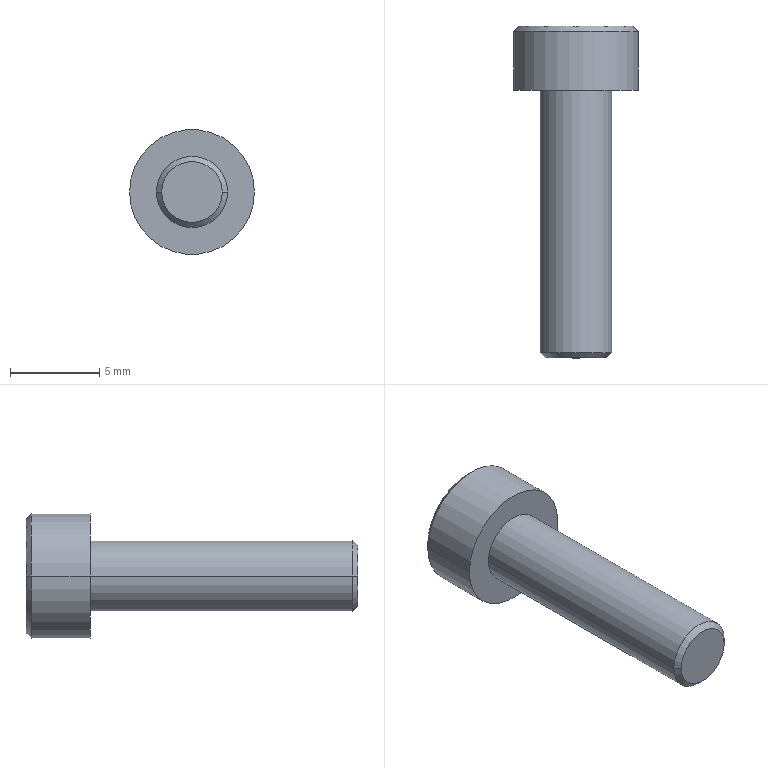Part | NX | 1 solid | 56 faces | box 7 x 18.6 x 7 mm | volume 309.592 mm3 | plane 44 | cone 6 | cylinder 6 | commonest cylinder face diameters 3 x2 4 x2 7 x2
STEP:
#1=CARTESIAN_POINT('',(1.7,-15.,0.));
#2=VERTEX_POINT('',#1);
#3=CARTESIAN_POINT('',(-1.7,-15.,0.));
#4=VERTEX_POINT('',#3);
#5=CARTESIAN_POINT('',(0.,-15.,0.));
#6=DIRECTION('',(0.,1.,0.));
#7=DIRECTION('',(-1.,0.,0.));
#8=AXIS2_PLACEMENT_3D('',#5,#6,#7);
#9=CIRCLE('',#8,1.7);
#10=EDGE_CURVE('',#2,#4,#9,.T.);
#11=ORIENTED_EDGE('',*,*,#10,.F.);
#12=CARTESIAN_POINT('',(0.,-15.,0.));
#13=DIRECTION('',(0.,1.,0.));
#14=DIRECTION('',(-1.,0.,0.));
#15=AXIS2_PLACEMENT_3D('',#12,#13,#14);
#16=CIRCLE('',#15,1.7);
#17=EDGE_CURVE('',#4,#2,#16,.T.);
#18=ORIENTED_EDGE('',*,*,#17,.F.);
#19=EDGE_LOOP('',(#11,#18));
#20=FACE_BOUND('',#19,.T.);
#21=CARTESIAN_POINT('',(0.,-15.,0.));
#22=DIRECTION('',(0.,-1.,0.));
#23=DIRECTION('',(0.,0.,-1.));
#24=AXIS2_PLACEMENT_3D('',#21,#22,#23);
#25=PLANE('',#24);
#26=ADVANCED_FACE('',(#20),#25,.T.);
#27=ORIENTED_EDGE('',*,*,#10,.T.);
#28=CARTESIAN_POINT('',(-2.,-14.7,0.));
#29=VERTEX_POINT('',#28);
#30=CARTESIAN_POINT('',(-1.85,-14.85,0.));
#31=DIRECTION('',(-0.7071,0.7071,0.));
#32=VECTOR('',#31,1000.);
#33=LINE('',#30,#32);
#34=EDGE_CURVE('',#29,#4,#33,.F.);
#35=ORIENTED_EDGE('',*,*,#34,.F.);
#36=CARTESIAN_POINT('',(2.,-14.7,0.));
#37=VERTEX_POINT('',#36);
#38=CARTESIAN_POINT('',(0.,-14.7,0.));
#39=DIRECTION('',(0.,1.,0.));
#40=DIRECTION('',(-1.,0.,0.));
#41=AXIS2_PLACEMENT_3D('',#38,#39,#40);
#42=CIRCLE('',#41,2.);
#43=EDGE_CURVE('',#37,#29,#42,.T.);
#44=ORIENTED_EDGE('',*,*,#43,.F.);
#45=CARTESIAN_POINT('',(1.85,-14.85,0.));
#46=DIRECTION('',(0.7071,0.7071,0.));
#47=VECTOR('',#46,1000.);
#48=LINE('',#45,#47);
#49=EDGE_CURVE('',#37,#2,#48,.F.);
#50=ORIENTED_EDGE('',*,*,#49,.T.);
#51=EDGE_LOOP('',(#27,#35,#44,#50));
#52=FACE_BOUND('',#51,.T.);
#53=CARTESIAN_POINT('',(0.,-14.85,0.));
#54=DIRECTION('',(0.,1.,0.));
#55=DIRECTION('',(1.,0.,0.));
#56=AXIS2_PLACEMENT_3D('',#53,#54,#55);
#57=CONICAL_SURFACE('',#56,1.85,0.7854);
#58=ADVANCED_FACE('',(#52),#57,.T.);
#59=CARTESIAN_POINT('',(0.,-14.7,0.));
#60=DIRECTION('',(0.,1.,0.));
#61=DIRECTION('',(-1.,0.,0.));
#62=AXIS2_PLACEMENT_3D('',#59,#60,#61);
#63=CIRCLE('',#62,2.);
#64=EDGE_CURVE('',#29,#37,#63,.T.);
#65=ORIENTED_EDGE('',*,*,#64,.T.);
#66=CARTESIAN_POINT('',(2.,0.,0.));
#67=VERTEX_POINT('',#66);
#68=CARTESIAN_POINT('',(2.,4.53,0.));
#69=DIRECTION('',(0.,-1.,0.));
#70=VECTOR('',#69,1000.);
#71=LINE('',#68,#70);
#72=EDGE_CURVE('',#67,#37,#71,.T.);
#73=ORIENTED_EDGE('',*,*,#72,.F.);
#74=CARTESIAN_POINT('',(-2.,0.,0.));
#75=VERTEX_POINT('',#74);
#76=CARTESIAN_POINT('',(0.,0.,0.));
#77=DIRECTION('',(0.,-1.,0.));
#78=DIRECTION('',(-1.,0.,0.));
#79=AXIS2_PLACEMENT_3D('',#76,#77,#78);
#80=CIRCLE('',#79,2.);
#81=EDGE_CURVE('',#67,#75,#80,.T.);
#82=ORIENTED_EDGE('',*,*,#81,.T.);
#83=CARTESIAN_POINT('',(-2.,4.53,0.));
#84=DIRECTION('',(0.,-1.,0.));
#85=VECTOR('',#84,1000.);
#86=LINE('',#83,#85);
#87=EDGE_CURVE('',#75,#29,#86,.T.);
#88=ORIENTED_EDGE('',*,*,#87,.T.);
#89=EDGE_LOOP('',(#65,#73,#82,#88));
#90=FACE_BOUND('',#89,.T.);
#91=CARTESIAN_POINT('',(0.,4.53,0.));
#92=DIRECTION('',(0.,-1.,0.));
#93=DIRECTION('',(-1.,0.,0.));
#94=AXIS2_PLACEMENT_3D('',#91,#92,#93);
#95=CYLINDRICAL_SURFACE('',#94,2.);
#96=ADVANCED_FACE('',(#90),#95,.T.);
#97=CARTESIAN_POINT('',(0.1875,3.6,1.945));
#98=VERTEX_POINT('',#97);
#99=CARTESIAN_POINT('',(0.4,3.6,1.702));
#100=VERTEX_POINT('',#99);
#101=CARTESIAN_POINT('',(0.1875,3.6,1.945));
#102=DIRECTION('',(0.659,0.,-0.7522));
#103=VECTOR('',#102,1000.);
#104=LINE('',#101,#103);
#105=EDGE_CURVE('',#98,#100,#104,.T.);
#106=ORIENTED_EDGE('',*,*,#105,.T.);
#107=CARTESIAN_POINT('',(0.4,3.55,1.702));
#108=VERTEX_POINT('',#107);
#109=CARTESIAN_POINT('',(0.4,3.55,1.702));
#110=DIRECTION('',(0.,1.,0.));
#111=VECTOR('',#110,1000.);
#112=LINE('',#109,#111);
#113=EDGE_CURVE('',#108,#100,#112,.T.);
#114=ORIENTED_EDGE('',*,*,#113,.F.);
#115=CARTESIAN_POINT('',(0.1875,3.55,1.945));
#116=VERTEX_POINT('',#115);
#117=CARTESIAN_POINT('',(0.4,3.55,1.702));
#118=DIRECTION('',(-0.659,0.,0.7522));
#119=VECTOR('',#118,1000.);
#120=LINE('',#117,#119);
#121=EDGE_CURVE('',#108,#116,#120,.T.);
#122=ORIENTED_EDGE('',*,*,#121,.T.);
#123=CARTESIAN_POINT('',(0.1875,3.55,1.945));
#124=DIRECTION('',(0.,1.,0.));
#125=VECTOR('',#124,1000.);
#126=LINE('',#123,#125);
#127=EDGE_CURVE('',#116,#98,#126,.T.);
#128=ORIENTED_EDGE('',*,*,#127,.T.);
#129=EDGE_LOOP('',(#106,#114,#122,#128));
#130=FACE_BOUND('',#129,.T.);
#131=CARTESIAN_POINT('',(0.1875,3.6,1.945));
#132=DIRECTION('',(0.7522,0.,0.659));
#133=DIRECTION('',(0.,-1.,0.));
#134=AXIS2_PLACEMENT_3D('',#131,#132,#133);
#135=PLANE('',#134);
#136=ADVANCED_FACE('',(#130),#135,.F.);
#137=ORIENTED_EDGE('',*,*,#105,.F.);
#138=CARTESIAN_POINT('',(0.4,3.6,1.945));
#139=VERTEX_POINT('',#138);
#140=CARTESIAN_POINT('',(0.1875,3.6,1.945));
#141=DIRECTION('',(1.,0.,0.));
#142=VECTOR('',#141,1000.);
#143=LINE('',#140,#142);
#144=EDGE_CURVE('',#98,#139,#143,.T.);
#145=ORIENTED_EDGE('',*,*,#144,.T.);
#146=CARTESIAN_POINT('',(0.4,3.6,1.945));
#147=DIRECTION('',(0.,0.,-1.));
#148=VECTOR('',#147,1000.);
#149=LINE('',#146,#148);
#150=EDGE_CURVE('',#139,#100,#149,.T.);
#151=ORIENTED_EDGE('',*,*,#150,.T.);
#152=EDGE_LOOP('',(#137,#145,#151));
#153=FACE_BOUND('',#152,.T.);
#154=CARTESIAN_POINT('',(0.,3.6,0.));
#155=DIRECTION('',(0.,-1.,0.));
#156=DIRECTION('',(0.,0.,-1.));
#157=AXIS2_PLACEMENT_3D('',#154,#155,#156);
#158=PLANE('',#157);
#159=ADVANCED_FACE('',(#153),#158,.F.);
#160=CARTESIAN_POINT('',(3.5,0.,0.));
#161=VERTEX_POINT('',#160);
#162=CARTESIAN_POINT('',(-3.5,0.,0.));
#163=VERTEX_POINT('',#162);
#164=CARTESIAN_POINT('',(0.,0.,0.));
#165=DIRECTION('',(0.,1.,0.));
#166=DIRECTION('',(-1.,0.,0.));
#167=AXIS2_PLACEMENT_3D('',#164,#165,#166);
#168=CIRCLE('',#167,3.5);
#169=EDGE_CURVE('',#161,#163,#168,.T.);
#170=ORIENTED_EDGE('',*,*,#169,.F.);
#171=CARTESIAN_POINT('',(0.,0.,0.));
#172=DIRECTION('',(0.,1.,0.));
#173=DIRECTION('',(-1.,0.,0.));
#174=AXIS2_PLACEMENT_3D('',#171,#172,#173);
#175=CIRCLE('',#174,3.5);
#176=EDGE_CURVE('',#163,#161,#175,.T.);
#177=ORIENTED_EDGE('',*,*,#176,.F.);
#178=EDGE_LOOP('',(#170,#177));
#179=FACE_BOUND('',#178,.T.);
#180=CARTESIAN_POINT('',(0.,0.,0.));
#181=DIRECTION('',(0.,-1.,0.));
#182=DIRECTION('',(-1.,0.,0.));
#183=AXIS2_PLACEMENT_3D('',#180,#181,#182);
#184=CIRCLE('',#183,2.);
#185=EDGE_CURVE('',#75,#67,#184,.T.);
#186=ORIENTED_EDGE('',*,*,#185,.F.);
#187=ORIENTED_EDGE('',*,*,#81,.F.);
#188=EDGE_LOOP('',(#186,#187));
#189=FACE_BOUND('',#188,.T.);
#190=CARTESIAN_POINT('',(0.,0.,0.));
#191=DIRECTION('',(0.,-1.,0.));
#192=DIRECTION('',(0.,0.,-1.));
#193=AXIS2_PLACEMENT_3D('',#190,#191,#192);
#194=PLANE('',#193);
#195=ADVANCED_FACE('',(#179,#189),#194,.T.);
#196=CARTESIAN_POINT('',(3.5,3.3,0.));
#197=VERTEX_POINT('',#196);
#198=CARTESIAN_POINT('',(-3.5,3.3,0.));
#199=VERTEX_POINT('',#198);
#200=CARTESIAN_POINT('',(0.,3.3,0.));
#201=DIRECTION('',(0.,-1.,0.));
#202=DIRECTION('',(-1.,0.,0.));
#203=AXIS2_PLACEMENT_3D('',#200,#201,#202);
#204=CIRCLE('',#203,3.5);
#205=EDGE_CURVE('',#197,#199,#204,.T.);
#206=ORIENTED_EDGE('',*,*,#205,.T.);
#207=CARTESIAN_POINT('',(-3.5,4.53,0.));
#208=DIRECTION('',(0.,-1.,0.));
#209=VECTOR('',#208,1000.);
#210=LINE('',#207,#209);
#211=EDGE_CURVE('',#163,#199,#210,.F.);
#212=ORIENTED_EDGE('',*,*,#211,.F.);
#213=ORIENTED_EDGE('',*,*,#176,.T.);
#214=CARTESIAN_POINT('',(3.5,4.53,0.));
#215=DIRECTION('',(0.,-1.,0.));
#216=VECTOR('',#215,1000.);
#217=LINE('',#214,#216);
#218=EDGE_CURVE('',#161,#197,#217,.F.);
#219=ORIENTED_EDGE('',*,*,#218,.T.);
#220=EDGE_LOOP('',(#206,#212,#213,#219));
#221=FACE_BOUND('',#220,.T.);
#222=CARTESIAN_POINT('',(0.,4.53,0.));
#223=DIRECTION('',(0.,-1.,0.));
#224=DIRECTION('',(-1.,0.,0.));
#225=AXIS2_PLACEMENT_3D('',#222,#223,#224);
#226=CYLINDRICAL_SURFACE('',#225,3.5);
#227=ADVANCED_FACE('',(#221),#226,.T.);
#228=CARTESIAN_POINT('',(0.1,3.55,1.945));
#229=VERTEX_POINT('',#228);
#230=CARTESIAN_POINT('',(0.4,3.55,1.6));
#231=VERTEX_POINT('',#230);
#232=CARTESIAN_POINT('',(0.1,3.55,1.945));
#233=DIRECTION('',(0.6565,0.,-0.7543));
#234=VECTOR('',#233,1000.);
#235=LINE('',#232,#234);
#236=EDGE_CURVE('',#229,#231,#235,.T.);
#237=ORIENTED_EDGE('',*,*,#236,.F.);
#238=CARTESIAN_POINT('',(0.1,3.55,2.021));
#239=VERTEX_POINT('',#238);
#240=CARTESIAN_POINT('',(0.1,3.55,2.021));
#241=DIRECTION('',(0.,0.,-1.));
#242=VECTOR('',#241,1000.);
#243=LINE('',#240,#242);
#244=EDGE_CURVE('',#239,#229,#243,.T.);
#245=ORIENTED_EDGE('',*,*,#244,.F.);
#246=CARTESIAN_POINT('',(0.4,3.55,2.021));
#247=VERTEX_POINT('',#246);
#248=CARTESIAN_POINT('',(0.4,3.55,2.021));
#249=DIRECTION('',(-1.,0.,0.));
#250=VECTOR('',#249,1000.);
#251=LINE('',#248,#250);
#252=EDGE_CURVE('',#247,#239,#251,.T.);
#253=ORIENTED_EDGE('',*,*,#252,.F.);
#254=CARTESIAN_POINT('',(0.4,3.55,2.2));
#255=VERTEX_POINT('',#254);
#256=CARTESIAN_POINT('',(0.4,3.55,2.2));
#257=DIRECTION('',(0.,0.,-1.));
#258=VECTOR('',#257,1000.);
#259=LINE('',#256,#258);
#260=EDGE_CURVE('',#255,#247,#259,.T.);
#261=ORIENTED_EDGE('',*,*,#260,.F.);
#262=CARTESIAN_POINT('',(0.475,3.55,2.2));
#263=VERTEX_POINT('',#262);
#264=CARTESIAN_POINT('',(0.475,3.55,2.2));
#265=DIRECTION('',(-1.,0.,0.));
#266=VECTOR('',#265,1000.);
#267=LINE('',#264,#266);
#268=EDGE_CURVE('',#263,#255,#267,.T.);
#269=ORIENTED_EDGE('',*,*,#268,.F.);
#270=CARTESIAN_POINT('',(0.475,3.55,2.021));
#271=VERTEX_POINT('',#270);
#272=CARTESIAN_POINT('',(0.475,3.55,2.021));
#273=DIRECTION('',(0.,0.,1.));
#274=VECTOR('',#273,1000.);
#275=LINE('',#272,#274);
#276=EDGE_CURVE('',#271,#263,#275,.T.);
#277=ORIENTED_EDGE('',*,*,#276,.F.);
#278=CARTESIAN_POINT('',(0.6,3.55,2.021));
#279=VERTEX_POINT('',#278);
#280=CARTESIAN_POINT('',(0.6,3.55,2.021));
#281=DIRECTION('',(-1.,0.,0.));
#282=VECTOR('',#281,1000.);
#283=LINE('',#280,#282);
#284=EDGE_CURVE('',#279,#271,#283,.T.);
#285=ORIENTED_EDGE('',*,*,#284,.F.);
#286=CARTESIAN_POINT('',(0.6,3.55,1.945));
#287=VERTEX_POINT('',#286);
#288=CARTESIAN_POINT('',(0.6,3.55,1.945));
#289=DIRECTION('',(0.,0.,1.));
#290=VECTOR('',#289,1000.);
#291=LINE('',#288,#290);
#292=EDGE_CURVE('',#287,#279,#291,.T.);
#293=ORIENTED_EDGE('',*,*,#292,.F.);
#294=CARTESIAN_POINT('',(0.475,3.55,1.945));
#295=VERTEX_POINT('',#294);
#296=CARTESIAN_POINT('',(0.475,3.55,1.945));
#297=DIRECTION('',(1.,0.,0.));
#298=VECTOR('',#297,1000.);
#299=LINE('',#296,#298);
#300=EDGE_CURVE('',#295,#287,#299,.T.);
#301=ORIENTED_EDGE('',*,*,#300,.F.);
#302=CARTESIAN_POINT('',(0.475,3.55,1.6));
#303=VERTEX_POINT('',#302);
#304=CARTESIAN_POINT('',(0.475,3.55,1.6));
#305=DIRECTION('',(0.,0.,1.));
#306=VECTOR('',#305,1000.);
#307=LINE('',#304,#306);
#308=EDGE_CURVE('',#303,#295,#307,.T.);
#309=ORIENTED_EDGE('',*,*,#308,.F.);
#310=CARTESIAN_POINT('',(0.4,3.55,1.6));
#311=DIRECTION('',(1.,0.,0.));
#312=VECTOR('',#311,1000.);
#313=LINE('',#310,#312);
#314=EDGE_CURVE('',#231,#303,#313,.T.);
#315=ORIENTED_EDGE('',*,*,#314,.F.);
#316=EDGE_LOOP('',(#237,#245,#253,#261,#269,#277,#285,#293,#301,#309,#315));
#317=FACE_BOUND('',#316,.T.);
#318=ORIENTED_EDGE('',*,*,#121,.F.);
#319=CARTESIAN_POINT('',(0.4,3.55,1.945));
#320=VERTEX_POINT('',#319);
#321=CARTESIAN_POINT('',(0.4,3.55,1.945));
#322=DIRECTION('',(0.,0.,-1.));
#323=VECTOR('',#322,1000.);
#324=LINE('',#321,#323);
#325=EDGE_CURVE('',#320,#108,#324,.T.);
#326=ORIENTED_EDGE('',*,*,#325,.F.);
#327=CARTESIAN_POINT('',(0.1875,3.55,1.945));
#328=DIRECTION('',(1.,0.,0.));
#329=VECTOR('',#328,1000.);
#330=LINE('',#327,#329);
#331=EDGE_CURVE('',#116,#320,#330,.T.);
#332=ORIENTED_EDGE('',*,*,#331,.F.);
#333=EDGE_LOOP('',(#318,#326,#332));
#334=FACE_BOUND('',#333,.T.);
#335=CARTESIAN_POINT('',(0.,3.55,0.));
#336=DIRECTION('',(0.,1.,0.));
#337=DIRECTION('',(1.,0.,0.));
#338=AXIS2_PLACEMENT_3D('',#335,#336,#337);
#339=PLANE('',#338);
#340=ADVANCED_FACE('',(#317,#334),#339,.T.);
#341=CARTESIAN_POINT('',(-3.2,3.6,0.));
#342=VERTEX_POINT('',#341);
#343=CARTESIAN_POINT('',(3.2,3.6,0.));
#344=VERTEX_POINT('',#343);
#345=CARTESIAN_POINT('',(0.,3.6,0.));
#346=DIRECTION('',(0.,-1.,0.));
#347=DIRECTION('',(-1.,0.,0.));
#348=AXIS2_PLACEMENT_3D('',#345,#346,#347);
#349=CIRCLE('',#348,3.2);
#350=EDGE_CURVE('',#342,#344,#349,.T.);
#351=ORIENTED_EDGE('',*,*,#350,.T.);
#352=CARTESIAN_POINT('',(3.35,3.45,0.));
#353=DIRECTION('',(0.7071,-0.7071,0.));
#354=VECTOR('',#353,1000.);
#355=LINE('',#352,#354);
#356=EDGE_CURVE('',#344,#197,#355,.T.);
#357=ORIENTED_EDGE('',*,*,#356,.T.);
#358=CARTESIAN_POINT('',(0.,3.3,0.));
#359=DIRECTION('',(0.,-1.,0.));
#360=DIRECTION('',(-1.,0.,0.));
#361=AXIS2_PLACEMENT_3D('',#358,#359,#360);
#362=CIRCLE('',#361,3.5);
#363=EDGE_CURVE('',#199,#197,#362,.T.);
#364=ORIENTED_EDGE('',*,*,#363,.F.);
#365=CARTESIAN_POINT('',(-3.35,3.45,0.));
#366=DIRECTION('',(-0.7071,-0.7071,0.));
#367=VECTOR('',#366,1000.);
#368=LINE('',#365,#367);
#369=EDGE_CURVE('',#342,#199,#368,.T.);
#370=ORIENTED_EDGE('',*,*,#369,.F.);
#371=EDGE_LOOP('',(#351,#357,#364,#370));
#372=FACE_BOUND('',#371,.T.);
#373=CARTESIAN_POINT('',(0.,3.45,0.));
#374=DIRECTION('',(0.,-1.,0.));
#375=DIRECTION('',(-1.,0.,0.));
#376=AXIS2_PLACEMENT_3D('',#373,#374,#375);
#377=CONICAL_SURFACE('',#376,3.35,0.7854);
#378=ADVANCED_FACE('',(#372),#377,.T.);
#379=ORIENTED_EDGE('',*,*,#350,.F.);
#380=CARTESIAN_POINT('',(0.,3.6,0.));
#381=DIRECTION('',(0.,-1.,0.));
#382=DIRECTION('',(-1.,0.,0.));
#383=AXIS2_PLACEMENT_3D('',#380,#381,#382);
#384=CIRCLE('',#383,3.2);
#385=EDGE_CURVE('',#344,#342,#384,.T.);
#386=ORIENTED_EDGE('',*,*,#385,.F.);
#387=EDGE_LOOP('',(#379,#386));
#388=FACE_BOUND('',#387,.T.);
#389=CARTESIAN_POINT('',(-0.075,3.6,2.2));
#390=VERTEX_POINT('',#389);
#391=CARTESIAN_POINT('',(-0.075,3.6,1.728));
#392=VERTEX_POINT('',#391);
#393=CARTESIAN_POINT('',(-0.075,3.6,2.2));
#394=DIRECTION('',(0.,0.,-1.));
#395=VECTOR('',#394,1000.);
#396=LINE('',#393,#395);
#397=EDGE_CURVE('',#390,#392,#396,.T.);
#398=ORIENTED_EDGE('',*,*,#397,.T.);
#399=CARTESIAN_POINT('',(-0.25,3.6,2.2));
#400=VERTEX_POINT('',#399);
#401=CARTESIAN_POINT('',(-0.25,3.6,2.2));
#402=DIRECTION('',(0.3474,0.,-0.9377));
#403=VECTOR('',#402,1000.);
#404=LINE('',#401,#403);
#405=EDGE_CURVE('',#400,#392,#404,.T.);
#406=ORIENTED_EDGE('',*,*,#405,.F.);
#407=CARTESIAN_POINT('',(-0.35,3.6,2.2));
#408=VERTEX_POINT('',#407);
#409=CARTESIAN_POINT('',(-0.25,3.6,2.2));
#410=DIRECTION('',(-1.,0.,0.));
#411=VECTOR('',#410,1000.);
#412=LINE('',#409,#411);
#413=EDGE_CURVE('',#400,#408,#412,.T.);
#414=ORIENTED_EDGE('',*,*,#413,.T.);
#415=CARTESIAN_POINT('',(-0.525,3.6,1.728));
#416=VERTEX_POINT('',#415);
#417=CARTESIAN_POINT('',(-0.525,3.6,1.728));
#418=DIRECTION('',(0.3474,0.,0.9377));
#419=VECTOR('',#418,1000.);
#420=LINE('',#417,#419);
#421=EDGE_CURVE('',#416,#408,#420,.T.);
#422=ORIENTED_EDGE('',*,*,#421,.F.);
#423=CARTESIAN_POINT('',(-0.525,3.6,2.2));
#424=VERTEX_POINT('',#423);
#425=CARTESIAN_POINT('',(-0.525,3.6,1.728));
#426=DIRECTION('',(0.,0.,1.));
#427=VECTOR('',#426,1000.);
#428=LINE('',#425,#427);
#429=EDGE_CURVE('',#416,#424,#428,.T.);
#430=ORIENTED_EDGE('',*,*,#429,.T.);
#431=CARTESIAN_POINT('',(-0.6,3.6,2.2));
#432=VERTEX_POINT('',#431);
#433=CARTESIAN_POINT('',(-0.525,3.6,2.2));
#434=DIRECTION('',(-1.,0.,0.));
#435=VECTOR('',#434,1000.);
#436=LINE('',#433,#435);
#437=EDGE_CURVE('',#424,#432,#436,.T.);
#438=ORIENTED_EDGE('',*,*,#437,.T.);
#439=CARTESIAN_POINT('',(-0.6,3.6,1.6));
#440=VERTEX_POINT('',#439);
#441=CARTESIAN_POINT('',(-0.6,3.6,2.2));
#442=DIRECTION('',(0.,0.,-1.));
#443=VECTOR('',#442,1000.);
#444=LINE('',#441,#443);
#445=EDGE_CURVE('',#432,#440,#444,.T.);
#446=ORIENTED_EDGE('',*,*,#445,.T.);
#447=CARTESIAN_POINT('',(-0.4875,3.6,1.6));
#448=VERTEX_POINT('',#447);
#449=CARTESIAN_POINT('',(-0.6,3.6,1.6));
#450=DIRECTION('',(1.,0.,0.));
#451=VECTOR('',#450,1000.);
#452=LINE('',#449,#451);
#453=EDGE_CURVE('',#440,#448,#452,.T.);
#454=ORIENTED_EDGE('',*,*,#453,.T.);
#455=CARTESIAN_POINT('',(-0.3,3.6,2.136));
#456=VERTEX_POINT('',#455);
#457=CARTESIAN_POINT('',(-0.3,3.6,2.136));
#458=DIRECTION('',(-0.3301,0.,-0.9439));
#459=VECTOR('',#458,1000.);
#460=LINE('',#457,#459);
#461=EDGE_CURVE('',#456,#448,#460,.T.);
#462=ORIENTED_EDGE('',*,*,#461,.F.);
#463=CARTESIAN_POINT('',(-0.132,3.6,1.656));
#464=VERTEX_POINT('',#463);
#465=CARTESIAN_POINT('',(-0.132,3.6,1.656));
#466=DIRECTION('',(-0.3301,0.,0.9439));
#467=VECTOR('',#466,1000.);
#468=LINE('',#465,#467);
#469=EDGE_CURVE('',#464,#456,#468,.T.);
#470=ORIENTED_EDGE('',*,*,#469,.F.);
#471=CARTESIAN_POINT('',(-1.5,3.6,0.866));
#472=VERTEX_POINT('',#471);
#473=CARTESIAN_POINT('',(-1.5,3.6,0.866));
#474=DIRECTION('',(0.866,0.,0.5));
#475=VECTOR('',#474,1000.);
#476=LINE('',#473,#475);
#477=EDGE_CURVE('',#472,#464,#476,.T.);
#478=ORIENTED_EDGE('',*,*,#477,.F.);
#479=CARTESIAN_POINT('',(-1.5,3.6,-0.866));
#480=VERTEX_POINT('',#479);
#481=CARTESIAN_POINT('',(-1.5,3.6,0.866));
#482=DIRECTION('',(0.,0.,-1.));
#483=VECTOR('',#482,1000.);
#484=LINE('',#481,#483);
#485=EDGE_CURVE('',#472,#480,#484,.T.);
#486=ORIENTED_EDGE('',*,*,#485,.T.);
#487=CARTESIAN_POINT('',(0.,3.6,-1.732));
#488=VERTEX_POINT('',#487);
#489=CARTESIAN_POINT('',(0.,3.6,-1.732));
#490=DIRECTION('',(-0.866,0.,0.5));
#491=VECTOR('',#490,1000.);
#492=LINE('',#489,#491);
#493=EDGE_CURVE('',#488,#480,#492,.T.);
#494=ORIENTED_EDGE('',*,*,#493,.F.);
#495=CARTESIAN_POINT('',(1.5,3.6,-0.866));
#496=VERTEX_POINT('',#495);
#497=CARTESIAN_POINT('',(1.5,3.6,-0.866));
#498=DIRECTION('',(-0.866,0.,-0.5));
#499=VECTOR('',#498,1000.);
#500=LINE('',#497,#499);
#501=EDGE_CURVE('',#496,#488,#500,.T.);
#502=ORIENTED_EDGE('',*,*,#501,.F.);
#503=CARTESIAN_POINT('',(1.5,3.6,0.866));
#504=VERTEX_POINT('',#503);
#505=CARTESIAN_POINT('',(1.5,3.6,-0.866));
#506=DIRECTION('',(0.,0.,1.));
#507=VECTOR('',#506,1000.);
#508=LINE('',#505,#507);
#509=EDGE_CURVE('',#496,#504,#508,.T.);
#510=ORIENTED_EDGE('',*,*,#509,.T.);
#511=CARTESIAN_POINT('',(0.,3.6,1.732));
#512=VERTEX_POINT('',#511);
#513=CARTESIAN_POINT('',(0.,3.6,1.732));
#514=DIRECTION('',(0.866,0.,-0.5));
#515=VECTOR('',#514,1000.);
#516=LINE('',#513,#515);
#517=EDGE_CURVE('',#512,#504,#516,.T.);
#518=ORIENTED_EDGE('',*,*,#517,.F.);
#519=CARTESIAN_POINT('',(0.,3.6,2.2));
#520=VERTEX_POINT('',#519);
#521=CARTESIAN_POINT('',(0.,3.6,1.732));
#522=DIRECTION('',(0.,0.,1.));
#523=VECTOR('',#522,1000.);
#524=LINE('',#521,#523);
#525=EDGE_CURVE('',#512,#520,#524,.T.);
#526=ORIENTED_EDGE('',*,*,#525,.T.);
#527=CARTESIAN_POINT('',(0.,3.6,2.2));
#528=DIRECTION('',(-1.,0.,0.));
#529=VECTOR('',#528,1000.);
#530=LINE('',#527,#529);
#531=EDGE_CURVE('',#520,#390,#530,.T.);
#532=ORIENTED_EDGE('',*,*,#531,.T.);
#533=EDGE_LOOP('',(#398,#406,#414,#422,#430,#438,#446,#454,#462,#470,#478,#486,#494,#502,#510,#518,#526,#532));
#534=FACE_BOUND('',#533,.T.);
#535=CARTESIAN_POINT('',(0.4,3.6,1.6));
#536=VERTEX_POINT('',#535);
#537=CARTESIAN_POINT('',(0.1,3.6,1.945));
#538=VERTEX_POINT('',#537);
#539=CARTESIAN_POINT('',(0.4,3.6,1.6));
#540=DIRECTION('',(-0.6565,0.,0.7543));
#541=VECTOR('',#540,1000.);
#542=LINE('',#539,#541);
#543=EDGE_CURVE('',#536,#538,#542,.T.);
#544=ORIENTED_EDGE('',*,*,#543,.F.);
#545=CARTESIAN_POINT('',(0.475,3.6,1.6));
#546=VERTEX_POINT('',#545);
#547=CARTESIAN_POINT('',(0.4,3.6,1.6));
#548=DIRECTION('',(1.,0.,0.));
#549=VECTOR('',#548,1000.);
#550=LINE('',#547,#549);
#551=EDGE_CURVE('',#536,#546,#550,.T.);
#552=ORIENTED_EDGE('',*,*,#551,.T.);
#553=CARTESIAN_POINT('',(0.475,3.6,1.945));
#554=VERTEX_POINT('',#553);
#555=CARTESIAN_POINT('',(0.475,3.6,1.6));
#556=DIRECTION('',(0.,0.,1.));
#557=VECTOR('',#556,1000.);
#558=LINE('',#555,#557);
#559=EDGE_CURVE('',#546,#554,#558,.T.);
#560=ORIENTED_EDGE('',*,*,#559,.T.);
#561=CARTESIAN_POINT('',(0.6,3.6,1.945));
#562=VERTEX_POINT('',#561);
#563=CARTESIAN_POINT('',(0.475,3.6,1.945));
#564=DIRECTION('',(1.,0.,0.));
#565=VECTOR('',#564,1000.);
#566=LINE('',#563,#565);
#567=EDGE_CURVE('',#554,#562,#566,.T.);
#568=ORIENTED_EDGE('',*,*,#567,.T.);
#569=CARTESIAN_POINT('',(0.6,3.6,2.021));
#570=VERTEX_POINT('',#569);
#571=CARTESIAN_POINT('',(0.6,3.6,1.945));
#572=DIRECTION('',(0.,0.,1.));
#573=VECTOR('',#572,1000.);
#574=LINE('',#571,#573);
#575=EDGE_CURVE('',#562,#570,#574,.T.);
#576=ORIENTED_EDGE('',*,*,#575,.T.);
#577=CARTESIAN_POINT('',(0.475,3.6,2.021));
#578=VERTEX_POINT('',#577);
#579=CARTESIAN_POINT('',(0.6,3.6,2.021));
#580=DIRECTION('',(-1.,0.,0.));
#581=VECTOR('',#580,1000.);
#582=LINE('',#579,#581);
#583=EDGE_CURVE('',#570,#578,#582,.T.);
#584=ORIENTED_EDGE('',*,*,#583,.T.);
#585=CARTESIAN_POINT('',(0.475,3.6,2.2));
#586=VERTEX_POINT('',#585);
#587=CARTESIAN_POINT('',(0.475,3.6,2.021));
#588=DIRECTION('',(0.,0.,1.));
#589=VECTOR('',#588,1000.);
#590=LINE('',#587,#589);
#591=EDGE_CURVE('',#578,#586,#590,.T.);
#592=ORIENTED_EDGE('',*,*,#591,.T.);
#593=CARTESIAN_POINT('',(0.4,3.6,2.2));
#594=VERTEX_POINT('',#593);
#595=CARTESIAN_POINT('',(0.475,3.6,2.2));
#596=DIRECTION('',(-1.,0.,0.));
#597=VECTOR('',#596,1000.);
#598=LINE('',#595,#597);
#599=EDGE_CURVE('',#586,#594,#598,.T.);
#600=ORIENTED_EDGE('',*,*,#599,.T.);
#601=CARTESIAN_POINT('',(0.4,3.6,2.021));
#602=VERTEX_POINT('',#601);
#603=CARTESIAN_POINT('',(0.4,3.6,2.2));
#604=DIRECTION('',(0.,0.,-1.));
#605=VECTOR('',#604,1000.);
#606=LINE('',#603,#605);
#607=EDGE_CURVE('',#594,#602,#606,.T.);
#608=ORIENTED_EDGE('',*,*,#607,.T.);
#609=CARTESIAN_POINT('',(0.1,3.6,2.021));
#610=VERTEX_POINT('',#609);
#611=CARTESIAN_POINT('',(0.4,3.6,2.021));
#612=DIRECTION('',(-1.,0.,0.));
#613=VECTOR('',#612,1000.);
#614=LINE('',#611,#613);
#615=EDGE_CURVE('',#602,#610,#614,.T.);
#616=ORIENTED_EDGE('',*,*,#615,.T.);
#617=CARTESIAN_POINT('',(0.1,3.6,2.021));
#618=DIRECTION('',(0.,0.,-1.));
#619=VECTOR('',#618,1000.);
#620=LINE('',#617,#619);
#621=EDGE_CURVE('',#610,#538,#620,.T.);
#622=ORIENTED_EDGE('',*,*,#621,.T.);
#623=EDGE_LOOP('',(#544,#552,#560,#568,#576,#584,#592,#600,#608,#616,#622));
#624=FACE_BOUND('',#623,.T.);
#625=CARTESIAN_POINT('',(0.,3.6,0.));
#626=DIRECTION('',(0.,-1.,0.));
#627=DIRECTION('',(0.,0.,-1.));
#628=AXIS2_PLACEMENT_3D('',#625,#626,#627);
#629=PLANE('',#628);
#630=ADVANCED_FACE('',(#388,#534,#624),#629,.F.);
#631=ORIENTED_EDGE('',*,*,#621,.F.);
#632=CARTESIAN_POINT('',(0.1,3.55,2.021));
#633=DIRECTION('',(0.,1.,0.));
#634=VECTOR('',#633,1000.);
#635=LINE('',#632,#634);
#636=EDGE_CURVE('',#239,#610,#635,.T.);
#637=ORIENTED_EDGE('',*,*,#636,.F.);
#638=ORIENTED_EDGE('',*,*,#244,.T.);
#639=CARTESIAN_POINT('',(0.1,3.55,1.945));
#640=DIRECTION('',(0.,1.,0.));
#641=VECTOR('',#640,1000.);
#642=LINE('',#639,#641);
#643=EDGE_CURVE('',#229,#538,#642,.T.);
#644=ORIENTED_EDGE('',*,*,#643,.T.);
#645=EDGE_LOOP('',(#631,#637,#638,#644));
#646=FACE_BOUND('',#645,.T.);
#647=CARTESIAN_POINT('',(0.1,3.6,1.945));
#648=DIRECTION('',(-1.,0.,0.));
#649=DIRECTION('',(0.,0.,1.));
#650=AXIS2_PLACEMENT_3D('',#647,#648,#649);
#651=PLANE('',#650);
#652=ADVANCED_FACE('',(#646),#651,.F.);
#653=ORIENTED_EDGE('',*,*,#397,.F.);
#654=CARTESIAN_POINT('',(-0.075,3.55,2.2));
#655=VERTEX_POINT('',#654);
#656=CARTESIAN_POINT('',(-0.075,3.55,2.2));
#657=DIRECTION('',(0.,1.,0.));
#658=VECTOR('',#657,1000.);
#659=LINE('',#656,#658);
#660=EDGE_CURVE('',#655,#390,#659,.T.);
#661=ORIENTED_EDGE('',*,*,#660,.F.);
#662=CARTESIAN_POINT('',(-0.075,3.55,1.728));
#663=VERTEX_POINT('',#662);
#664=CARTESIAN_POINT('',(-0.075,3.55,2.2));
#665=DIRECTION('',(0.,0.,-1.));
#666=VECTOR('',#665,1000.);
#667=LINE('',#664,#666);
#668=EDGE_CURVE('',#655,#663,#667,.T.);
#669=ORIENTED_EDGE('',*,*,#668,.T.);
#670=CARTESIAN_POINT('',(-0.075,3.55,1.728));
#671=DIRECTION('',(0.,1.,0.));
#672=VECTOR('',#671,1000.);
#673=LINE('',#670,#672);
#674=EDGE_CURVE('',#663,#392,#673,.T.);
#675=ORIENTED_EDGE('',*,*,#674,.T.);
#676=EDGE_LOOP('',(#653,#661,#669,#675));
#677=FACE_BOUND('',#676,.T.);
#678=CARTESIAN_POINT('',(-0.075,3.6,1.728));
#679=DIRECTION('',(-1.,0.,0.));
#680=DIRECTION('',(0.,0.,1.));
#681=AXIS2_PLACEMENT_3D('',#678,#679,#680);
#682=PLANE('',#681);
#683=ADVANCED_FACE('',(#677),#682,.F.);
#684=ORIENTED_EDGE('',*,*,#405,.T.);
#685=ORIENTED_EDGE('',*,*,#674,.F.);
#686=CARTESIAN_POINT('',(-0.25,3.55,2.2));
#687=VERTEX_POINT('',#686);
#688=CARTESIAN_POINT('',(-0.075,3.55,1.728));
#689=DIRECTION('',(-0.3474,0.,0.9377));
#690=VECTOR('',#689,1000.);
#691=LINE('',#688,#690);
#692=EDGE_CURVE('',#663,#687,#691,.T.);
#693=ORIENTED_EDGE('',*,*,#692,.T.);
#694=CARTESIAN_POINT('',(-0.25,3.55,2.2));
#695=DIRECTION('',(0.,1.,0.));
#696=VECTOR('',#695,1000.);
#697=LINE('',#694,#696);
#698=EDGE_CURVE('',#687,#400,#697,.T.);
#699=ORIENTED_EDGE('',*,*,#698,.T.);
#700=EDGE_LOOP('',(#684,#685,#693,#699));
#701=FACE_BOUND('',#700,.T.);
#702=CARTESIAN_POINT('',(-0.25,3.6,2.2));
#703=DIRECTION('',(0.9377,0.,0.3474));
#704=DIRECTION('',(0.,-1.,0.));
#705=AXIS2_PLACEMENT_3D('',#702,#703,#704);
#706=PLANE('',#705);
#707=ADVANCED_FACE('',(#701),#706,.F.);
#708=ORIENTED_EDGE('',*,*,#413,.F.);
#709=ORIENTED_EDGE('',*,*,#698,.F.);
#710=CARTESIAN_POINT('',(-0.35,3.55,2.2));
#711=VERTEX_POINT('',#710);
#712=CARTESIAN_POINT('',(-0.25,3.55,2.2));
#713=DIRECTION('',(-1.,0.,0.));
#714=VECTOR('',#713,1000.);
#715=LINE('',#712,#714);
#716=EDGE_CURVE('',#687,#711,#715,.T.);
#717=ORIENTED_EDGE('',*,*,#716,.T.);
#718=CARTESIAN_POINT('',(-0.35,3.55,2.2));
#719=DIRECTION('',(0.,1.,0.));
#720=VECTOR('',#719,1000.);
#721=LINE('',#718,#720);
#722=EDGE_CURVE('',#711,#408,#721,.T.);
#723=ORIENTED_EDGE('',*,*,#722,.T.);
#724=EDGE_LOOP('',(#708,#709,#717,#723));
#725=FACE_BOUND('',#724,.T.);
#726=CARTESIAN_POINT('',(-0.35,3.6,2.2));
#727=DIRECTION('',(0.,0.,1.));
#728=DIRECTION('',(1.,0.,0.));
#729=AXIS2_PLACEMENT_3D('',#726,#727,#728);
#730=PLANE('',#729);
#731=ADVANCED_FACE('',(#725),#730,.F.);
#732=ORIENTED_EDGE('',*,*,#421,.T.);
#733=ORIENTED_EDGE('',*,*,#722,.F.);
#734=CARTESIAN_POINT('',(-0.525,3.55,1.728));
#735=VERTEX_POINT('',#734);
#736=CARTESIAN_POINT('',(-0.35,3.55,2.2));
#737=DIRECTION('',(-0.3474,0.,-0.9377));
#738=VECTOR('',#737,1000.);
#739=LINE('',#736,#738);
#740=EDGE_CURVE('',#711,#735,#739,.T.);
#741=ORIENTED_EDGE('',*,*,#740,.T.);
#742=CARTESIAN_POINT('',(-0.525,3.55,1.728));
#743=DIRECTION('',(0.,1.,0.));
#744=VECTOR('',#743,1000.);
#745=LINE('',#742,#744);
#746=EDGE_CURVE('',#735,#416,#745,.T.);
#747=ORIENTED_EDGE('',*,*,#746,.T.);
#748=EDGE_LOOP('',(#732,#733,#741,#747));
#749=FACE_BOUND('',#748,.T.);
#750=CARTESIAN_POINT('',(-0.525,3.6,1.728));
#751=DIRECTION('',(-0.9377,0.,0.3474));
#752=DIRECTION('',(0.,1.,0.));
#753=AXIS2_PLACEMENT_3D('',#750,#751,#752);
#754=PLANE('',#753);
#755=ADVANCED_FACE('',(#749),#754,.F.);
#756=ORIENTED_EDGE('',*,*,#429,.F.);
#757=ORIENTED_EDGE('',*,*,#746,.F.);
#758=CARTESIAN_POINT('',(-0.525,3.55,2.2));
#759=VERTEX_POINT('',#758);
#760=CARTESIAN_POINT('',(-0.525,3.55,1.728));
#761=DIRECTION('',(0.,0.,1.));
#762=VECTOR('',#761,1000.);
#763=LINE('',#760,#762);
#764=EDGE_CURVE('',#735,#759,#763,.T.);
#765=ORIENTED_EDGE('',*,*,#764,.T.);
#766=CARTESIAN_POINT('',(-0.525,3.55,2.2));
#767=DIRECTION('',(0.,1.,0.));
#768=VECTOR('',#767,1000.);
#769=LINE('',#766,#768);
#770=EDGE_CURVE('',#759,#424,#769,.T.);
#771=ORIENTED_EDGE('',*,*,#770,.T.);
#772=EDGE_LOOP('',(#756,#757,#765,#771));
#773=FACE_BOUND('',#772,.T.);
#774=CARTESIAN_POINT('',(-0.525,3.6,2.2));
#775=DIRECTION('',(1.,0.,0.));
#776=DIRECTION('',(0.,1.,0.));
#777=AXIS2_PLACEMENT_3D('',#774,#775,#776);
#778=PLANE('',#777);
#779=ADVANCED_FACE('',(#773),#778,.F.);
#780=ORIENTED_EDGE('',*,*,#437,.F.);
#781=ORIENTED_EDGE('',*,*,#770,.F.);
#782=CARTESIAN_POINT('',(-0.6,3.55,2.2));
#783=VERTEX_POINT('',#782);
#784=CARTESIAN_POINT('',(-0.525,3.55,2.2));
#785=DIRECTION('',(-1.,0.,0.));
#786=VECTOR('',#785,1000.);
#787=LINE('',#784,#786);
#788=EDGE_CURVE('',#759,#783,#787,.T.);
#789=ORIENTED_EDGE('',*,*,#788,.T.);
#790=CARTESIAN_POINT('',(-0.6,3.55,2.2));
#791=DIRECTION('',(0.,1.,0.));
#792=VECTOR('',#791,1000.);
#793=LINE('',#790,#792);
#794=EDGE_CURVE('',#783,#432,#793,.T.);
#795=ORIENTED_EDGE('',*,*,#794,.T.);
#796=EDGE_LOOP('',(#780,#781,#789,#795));
#797=FACE_BOUND('',#796,.T.);
#798=CARTESIAN_POINT('',(-0.6,3.6,2.2));
#799=DIRECTION('',(0.,0.,1.));
#800=DIRECTION('',(1.,0.,0.));
#801=AXIS2_PLACEMENT_3D('',#798,#799,#800);
#802=PLANE('',#801);
#803=ADVANCED_FACE('',(#797),#802,.F.);
#804=ORIENTED_EDGE('',*,*,#445,.F.);
#805=ORIENTED_EDGE('',*,*,#794,.F.);
#806=CARTESIAN_POINT('',(-0.6,3.55,1.6));
#807=VERTEX_POINT('',#806);
#808=CARTESIAN_POINT('',(-0.6,3.55,2.2));
#809=DIRECTION('',(0.,0.,-1.));
#810=VECTOR('',#809,1000.);
#811=LINE('',#808,#810);
#812=EDGE_CURVE('',#783,#807,#811,.T.);
#813=ORIENTED_EDGE('',*,*,#812,.T.);
#814=CARTESIAN_POINT('',(-0.6,3.55,1.6));
#815=DIRECTION('',(0.,1.,0.));
#816=VECTOR('',#815,1000.);
#817=LINE('',#814,#816);
#818=EDGE_CURVE('',#807,#440,#817,.T.);
#819=ORIENTED_EDGE('',*,*,#818,.T.);
#820=EDGE_LOOP('',(#804,#805,#813,#819));
#821=FACE_BOUND('',#820,.T.);
#822=CARTESIAN_POINT('',(-0.6,3.6,1.6));
#823=DIRECTION('',(-1.,0.,0.));
#824=DIRECTION('',(0.,0.,1.));
#825=AXIS2_PLACEMENT_3D('',#822,#823,#824);
#826=PLANE('',#825);
#827=ADVANCED_FACE('',(#821),#826,.F.);
#828=ORIENTED_EDGE('',*,*,#453,.F.);
#829=ORIENTED_EDGE('',*,*,#818,.F.);
#830=CARTESIAN_POINT('',(-0.4875,3.55,1.6));
#831=VERTEX_POINT('',#830);
#832=CARTESIAN_POINT('',(-0.6,3.55,1.6));
#833=DIRECTION('',(1.,0.,0.));
#834=VECTOR('',#833,1000.);
#835=LINE('',#832,#834);
#836=EDGE_CURVE('',#807,#831,#835,.T.);
#837=ORIENTED_EDGE('',*,*,#836,.T.);
#838=CARTESIAN_POINT('',(-0.4875,3.55,1.6));
#839=DIRECTION('',(0.,1.,0.));
#840=VECTOR('',#839,1000.);
#841=LINE('',#838,#840);
#842=EDGE_CURVE('',#831,#448,#841,.T.);
#843=ORIENTED_EDGE('',*,*,#842,.T.);
#844=EDGE_LOOP('',(#828,#829,#837,#843));
#845=FACE_BOUND('',#844,.T.);
#846=CARTESIAN_POINT('',(-0.4875,3.6,1.6));
#847=DIRECTION('',(0.,0.,-1.));
#848=DIRECTION('',(0.,-1.,0.));
#849=AXIS2_PLACEMENT_3D('',#846,#847,#848);
#850=PLANE('',#849);
#851=ADVANCED_FACE('',(#845),#850,.F.);
#852=ORIENTED_EDGE('',*,*,#461,.T.);
#853=ORIENTED_EDGE('',*,*,#842,.F.);
#854=CARTESIAN_POINT('',(-0.3,3.55,2.136));
#855=VERTEX_POINT('',#854);
#856=CARTESIAN_POINT('',(-0.4875,3.55,1.6));
#857=DIRECTION('',(0.3301,0.,0.9439));
#858=VECTOR('',#857,1000.);
#859=LINE('',#856,#858);
#860=EDGE_CURVE('',#831,#855,#859,.T.);
#861=ORIENTED_EDGE('',*,*,#860,.T.);
#862=CARTESIAN_POINT('',(-0.3,3.55,2.136));
#863=DIRECTION('',(0.,1.,0.));
#864=VECTOR('',#863,1000.);
#865=LINE('',#862,#864);
#866=EDGE_CURVE('',#855,#456,#865,.T.);
#867=ORIENTED_EDGE('',*,*,#866,.T.);
#868=EDGE_LOOP('',(#852,#853,#861,#867));
#869=FACE_BOUND('',#868,.T.);
#870=CARTESIAN_POINT('',(-0.3,3.6,2.136));
#871=DIRECTION('',(0.9439,0.,-0.3301));
#872=DIRECTION('',(0.,-1.,0.));
#873=AXIS2_PLACEMENT_3D('',#870,#871,#872);
#874=PLANE('',#873);
#875=ADVANCED_FACE('',(#869),#874,.F.);
#876=ORIENTED_EDGE('',*,*,#469,.T.);
#877=ORIENTED_EDGE('',*,*,#866,.F.);
#878=CARTESIAN_POINT('',(-0.132,3.55,1.656));
#879=VERTEX_POINT('',#878);
#880=CARTESIAN_POINT('',(-0.3,3.55,2.136));
#881=DIRECTION('',(0.3301,0.,-0.9439));
#882=VECTOR('',#881,1000.);
#883=LINE('',#880,#882);
#884=EDGE_CURVE('',#855,#879,#883,.T.);
#885=ORIENTED_EDGE('',*,*,#884,.T.);
#886=CARTESIAN_POINT('',(-0.132,3.55,1.656));
#887=DIRECTION('',(0.,1.,0.));
#888=VECTOR('',#887,1000.);
#889=LINE('',#886,#888);
#890=EDGE_CURVE('',#879,#464,#889,.T.);
#891=ORIENTED_EDGE('',*,*,#890,.T.);
#892=EDGE_LOOP('',(#876,#877,#885,#891));
#893=FACE_BOUND('',#892,.T.);
#894=CARTESIAN_POINT('',(-0.1125,3.6,1.6));
#895=DIRECTION('',(-0.9439,0.,-0.3301));
#896=DIRECTION('',(-0.3301,0.,0.9439));
#897=AXIS2_PLACEMENT_3D('',#894,#895,#896);
#898=PLANE('',#897);
#899=ADVANCED_FACE('',(#893),#898,.F.);
#900=CARTESIAN_POINT('',(0.,3.55,1.732));
#901=VERTEX_POINT('',#900);
#902=CARTESIAN_POINT('',(-0.132,3.55,1.656));
#903=DIRECTION('',(0.866,0.,0.5));
#904=VECTOR('',#903,1000.);
#905=LINE('',#902,#904);
#906=EDGE_CURVE('',#879,#901,#905,.T.);
#907=ORIENTED_EDGE('',*,*,#906,.T.);
#908=CARTESIAN_POINT('',(0.,2.1,1.732));
#909=VERTEX_POINT('',#908);
#910=CARTESIAN_POINT('',(0.,2.1,1.732));
#911=DIRECTION('',(0.,1.,0.));
#912=VECTOR('',#911,1000.);
#913=LINE('',#910,#912);
#914=EDGE_CURVE('',#909,#901,#913,.T.);
#915=ORIENTED_EDGE('',*,*,#914,.F.);
#916=CARTESIAN_POINT('',(-0.75,2.1,1.299));
#917=VERTEX_POINT('',#916);
#918=CARTESIAN_POINT('',(0.,2.1,1.732));
#919=DIRECTION('',(-0.866,0.,-0.5));
#920=VECTOR('',#919,1000.);
#921=LINE('',#918,#920);
#922=EDGE_CURVE('',#909,#917,#921,.T.);
#923=ORIENTED_EDGE('',*,*,#922,.T.);
#924=CARTESIAN_POINT('',(-1.5,2.1,0.866));
#925=VERTEX_POINT('',#924);
#926=CARTESIAN_POINT('',(-0.75,2.1,1.299));
#927=DIRECTION('',(-0.866,0.,-0.5));
#928=VECTOR('',#927,1000.);
#929=LINE('',#926,#928);
#930=EDGE_CURVE('',#917,#925,#929,.T.);
#931=ORIENTED_EDGE('',*,*,#930,.T.);
#932=CARTESIAN_POINT('',(-1.5,2.1,0.866));
#933=DIRECTION('',(0.,1.,0.));
#934=VECTOR('',#933,1000.);
#935=LINE('',#932,#934);
#936=EDGE_CURVE('',#925,#472,#935,.T.);
#937=ORIENTED_EDGE('',*,*,#936,.T.);
#938=ORIENTED_EDGE('',*,*,#477,.T.);
#939=ORIENTED_EDGE('',*,*,#890,.F.);
#940=EDGE_LOOP('',(#907,#915,#923,#931,#937,#938,#939));
#941=FACE_BOUND('',#940,.T.);
#942=CARTESIAN_POINT('',(-1.5,3.6,0.866));
#943=DIRECTION('',(-0.5,0.,0.866));
#944=DIRECTION('',(0.,1.,0.));
#945=AXIS2_PLACEMENT_3D('',#942,#943,#944);
#946=PLANE('',#945);
#947=ADVANCED_FACE('',(#941),#946,.F.);
#948=ORIENTED_EDGE('',*,*,#906,.F.);
#949=ORIENTED_EDGE('',*,*,#884,.F.);
#950=ORIENTED_EDGE('',*,*,#860,.F.);
#951=ORIENTED_EDGE('',*,*,#836,.F.);
#952=ORIENTED_EDGE('',*,*,#812,.F.);
#953=ORIENTED_EDGE('',*,*,#788,.F.);
#954=ORIENTED_EDGE('',*,*,#764,.F.);
#955=ORIENTED_EDGE('',*,*,#740,.F.);
#956=ORIENTED_EDGE('',*,*,#716,.F.);
#957=ORIENTED_EDGE('',*,*,#692,.F.);
#958=ORIENTED_EDGE('',*,*,#668,.F.);
#959=CARTESIAN_POINT('',(0.,3.55,2.2));
#960=VERTEX_POINT('',#959);
#961=CARTESIAN_POINT('',(0.,3.55,2.2));
#962=DIRECTION('',(-1.,0.,0.));
#963=VECTOR('',#962,1000.);
#964=LINE('',#961,#963);
#965=EDGE_CURVE('',#960,#655,#964,.T.);
#966=ORIENTED_EDGE('',*,*,#965,.F.);
#967=CARTESIAN_POINT('',(0.,3.55,1.732));
#968=DIRECTION('',(0.,0.,1.));
#969=VECTOR('',#968,1000.);
#970=LINE('',#967,#969);
#971=EDGE_CURVE('',#901,#960,#970,.T.);
#972=ORIENTED_EDGE('',*,*,#971,.F.);
#973=EDGE_LOOP('',(#948,#949,#950,#951,#952,#953,#954,#955,#956,#957,#958,#966,#972));
#974=FACE_BOUND('',#973,.T.);
#975=CARTESIAN_POINT('',(0.,3.55,0.));
#976=DIRECTION('',(0.,1.,0.));
#977=DIRECTION('',(1.,0.,0.));
#978=AXIS2_PLACEMENT_3D('',#975,#976,#977);
#979=PLANE('',#978);
#980=ADVANCED_FACE('',(#974),#979,.T.);
#981=ORIENTED_EDGE('',*,*,#525,.F.);
#982=CARTESIAN_POINT('',(0.,3.55,1.732));
#983=DIRECTION('',(0.,1.,0.));
#984=VECTOR('',#983,1000.);
#985=LINE('',#982,#984);
#986=EDGE_CURVE('',#901,#512,#985,.T.);
#987=ORIENTED_EDGE('',*,*,#986,.F.);
#988=ORIENTED_EDGE('',*,*,#971,.T.);
#989=CARTESIAN_POINT('',(0.,3.55,2.2));
#990=DIRECTION('',(0.,1.,0.));
#991=VECTOR('',#990,1000.);
#992=LINE('',#989,#991);
#993=EDGE_CURVE('',#960,#520,#992,.T.);
#994=ORIENTED_EDGE('',*,*,#993,.T.);
#995=EDGE_LOOP('',(#981,#987,#988,#994));
#996=FACE_BOUND('',#995,.T.);
#997=CARTESIAN_POINT('',(0.,3.6,2.2));
#998=DIRECTION('',(1.,0.,0.));
#999=DIRECTION('',(0.,1.,0.));
#1000=AXIS2_PLACEMENT_3D('',#997,#998,#999);
#1001=PLANE('',#1000);
#1002=ADVANCED_FACE('',(#996),#1001,.F.);
#1003=ORIENTED_EDGE('',*,*,#531,.F.);
#1004=ORIENTED_EDGE('',*,*,#993,.F.);
#1005=ORIENTED_EDGE('',*,*,#965,.T.);
#1006=ORIENTED_EDGE('',*,*,#660,.T.);
#1007=EDGE_LOOP('',(#1003,#1004,#1005,#1006));
#1008=FACE_BOUND('',#1007,.T.);
#1009=CARTESIAN_POINT('',(-0.075,3.6,2.2));
#1010=DIRECTION('',(0.,0.,1.));
#1011=DIRECTION('',(1.,0.,0.));
#1012=AXIS2_PLACEMENT_3D('',#1009,#1010,#1011);
#1013=PLANE('',#1012);
#1014=ADVANCED_FACE('',(#1008),#1013,.F.);
#1015=ORIENTED_EDGE('',*,*,#986,.T.);
#1016=ORIENTED_EDGE('',*,*,#517,.T.);
#1017=CARTESIAN_POINT('',(1.5,2.1,0.866));
#1018=VERTEX_POINT('',#1017);
#1019=CARTESIAN_POINT('',(1.5,2.1,0.866));
#1020=DIRECTION('',(0.,1.,0.));
#1021=VECTOR('',#1020,1000.);
#1022=LINE('',#1019,#1021);
#1023=EDGE_CURVE('',#1018,#504,#1022,.T.);
#1024=ORIENTED_EDGE('',*,*,#1023,.F.);
#1025=CARTESIAN_POINT('',(0.75,2.1,1.299));
#1026=VERTEX_POINT('',#1025);
#1027=CARTESIAN_POINT('',(1.5,2.1,0.866));
#1028=DIRECTION('',(-0.866,0.,0.5));
#1029=VECTOR('',#1028,1000.);
#1030=LINE('',#1027,#1029);
#1031=EDGE_CURVE('',#1018,#1026,#1030,.T.);
#1032=ORIENTED_EDGE('',*,*,#1031,.T.);
#1033=CARTESIAN_POINT('',(0.75,2.1,1.299));
#1034=DIRECTION('',(-0.866,0.,0.5));
#1035=VECTOR('',#1034,1000.);
#1036=LINE('',#1033,#1035);
#1037=EDGE_CURVE('',#1026,#909,#1036,.T.);
#1038=ORIENTED_EDGE('',*,*,#1037,.T.);
#1039=ORIENTED_EDGE('',*,*,#914,.T.);
#1040=EDGE_LOOP('',(#1015,#1016,#1024,#1032,#1038,#1039));
#1041=FACE_BOUND('',#1040,.T.);
#1042=CARTESIAN_POINT('',(0.,3.6,1.732));
#1043=DIRECTION('',(0.5,0.,0.866));
#1044=DIRECTION('',(0.,-1.,0.));
#1045=AXIS2_PLACEMENT_3D('',#1042,#1043,#1044);
#1046=PLANE('',#1045);
#1047=ADVANCED_FACE('',(#1041),#1046,.F.);
#1048=ORIENTED_EDGE('',*,*,#922,.F.);
#1049=ORIENTED_EDGE('',*,*,#1037,.F.);
#1050=CARTESIAN_POINT('',(0.,2.1,0.));
#1051=DIRECTION('',(0.,1.,0.));
#1052=DIRECTION('',(-0.5,0.,0.866));
#1053=AXIS2_PLACEMENT_3D('',#1050,#1051,#1052);
#1054=CIRCLE('',#1053,1.5);
#1055=EDGE_CURVE('',#917,#1026,#1054,.T.);
#1056=ORIENTED_EDGE('',*,*,#1055,.F.);
#1057=EDGE_LOOP('',(#1048,#1049,#1056));
#1058=FACE_BOUND('',#1057,.T.);
#1059=CARTESIAN_POINT('',(0.,2.1,0.));
#1060=DIRECTION('',(0.,1.,0.));
#1061=DIRECTION('',(1.,0.,0.));
#1062=AXIS2_PLACEMENT_3D('',#1059,#1060,#1061);
#1063=PLANE('',#1062);
#1064=ADVANCED_FACE('',(#1058),#1063,.T.);
#1065=CARTESIAN_POINT('',(-0.75,2.1,-1.299));
#1066=VERTEX_POINT('',#1065);
#1067=CARTESIAN_POINT('',(-1.5,2.1,0.));
#1068=VERTEX_POINT('',#1067);
#1069=CARTESIAN_POINT('',(0.,2.1,0.));
#1070=DIRECTION('',(0.,1.,0.));
#1071=DIRECTION('',(-0.5,0.,-0.866));
#1072=AXIS2_PLACEMENT_3D('',#1069,#1070,#1071);
#1073=CIRCLE('',#1072,1.5);
#1074=EDGE_CURVE('',#1066,#1068,#1073,.T.);
#1075=ORIENTED_EDGE('',*,*,#1074,.T.);
#1076=CARTESIAN_POINT('',(-1.5,1.8,0.));
#1077=VERTEX_POINT('',#1076);
#1078=CARTESIAN_POINT('',(-1.5,4.53,0.));
#1079=DIRECTION('',(0.,-1.,0.));
#1080=VECTOR('',#1079,1000.);
#1081=LINE('',#1078,#1080);
#1082=EDGE_CURVE('',#1077,#1068,#1081,.F.);
#1083=ORIENTED_EDGE('',*,*,#1082,.F.);
#1084=CARTESIAN_POINT('',(1.5,1.8,0.));
#1085=VERTEX_POINT('',#1084);
#1086=CARTESIAN_POINT('',(0.,1.8,0.));
#1087=DIRECTION('',(0.,-1.,0.));
#1088=DIRECTION('',(1.,0.,0.));
#1089=AXIS2_PLACEMENT_3D('',#1086,#1087,#1088);
#1090=CIRCLE('',#1089,1.5);
#1091=EDGE_CURVE('',#1077,#1085,#1090,.T.);
#1092=ORIENTED_EDGE('',*,*,#1091,.T.);
#1093=CARTESIAN_POINT('',(1.5,2.1,0.));
#1094=VERTEX_POINT('',#1093);
#1095=CARTESIAN_POINT('',(1.5,4.53,0.));
#1096=DIRECTION('',(0.,-1.,0.));
#1097=VECTOR('',#1096,1000.);
#1098=LINE('',#1095,#1097);
#1099=EDGE_CURVE('',#1085,#1094,#1098,.F.);
#1100=ORIENTED_EDGE('',*,*,#1099,.T.);
#1101=CARTESIAN_POINT('',(0.75,2.1,-1.299));
#1102=VERTEX_POINT('',#1101);
#1103=CARTESIAN_POINT('',(0.,2.1,0.));
#1104=DIRECTION('',(0.,1.,0.));
#1105=DIRECTION('',(1.,0.,0.));
#1106=AXIS2_PLACEMENT_3D('',#1103,#1104,#1105);
#1107=CIRCLE('',#1106,1.5);
#1108=EDGE_CURVE('',#1094,#1102,#1107,.T.);
#1109=ORIENTED_EDGE('',*,*,#1108,.T.);
#1110=CARTESIAN_POINT('',(0.,2.1,0.));
#1111=DIRECTION('',(0.,1.,0.));
#1112=DIRECTION('',(0.5,0.,-0.866));
#1113=AXIS2_PLACEMENT_3D('',#1110,#1111,#1112);
#1114=CIRCLE('',#1113,1.5);
#1115=EDGE_CURVE('',#1102,#1066,#1114,.T.);
#1116=ORIENTED_EDGE('',*,*,#1115,.T.);
#1117=EDGE_LOOP('',(#1075,#1083,#1092,#1100,#1109,#1116));
#1118=FACE_BOUND('',#1117,.T.);
#1119=CARTESIAN_POINT('',(0.,4.53,0.));
#1120=DIRECTION('',(0.,-1.,0.));
#1121=DIRECTION('',(-1.,0.,0.));
#1122=AXIS2_PLACEMENT_3D('',#1119,#1120,#1121);
#1123=CYLINDRICAL_SURFACE('',#1122,1.5);
#1124=ADVANCED_FACE('',(#1118),#1123,.F.);
#1125=CARTESIAN_POINT('',(1.5,2.1,0.));
#1126=DIRECTION('',(0.,0.,1.));
#1127=VECTOR('',#1126,1000.);
#1128=LINE('',#1125,#1127);
#1129=EDGE_CURVE('',#1094,#1018,#1128,.T.);
#1130=ORIENTED_EDGE('',*,*,#1129,.F.);
#1131=CARTESIAN_POINT('',(0.,2.1,0.));
#1132=DIRECTION('',(0.,1.,0.));
#1133=DIRECTION('',(0.5,0.,0.866));
#1134=AXIS2_PLACEMENT_3D('',#1131,#1132,#1133);
#1135=CIRCLE('',#1134,1.5);
#1136=EDGE_CURVE('',#1026,#1094,#1135,.T.);
#1137=ORIENTED_EDGE('',*,*,#1136,.F.);
#1138=ORIENTED_EDGE('',*,*,#1031,.F.);
#1139=EDGE_LOOP('',(#1130,#1137,#1138));
#1140=FACE_BOUND('',#1139,.T.);
#1141=CARTESIAN_POINT('',(0.,2.1,0.));
#1142=DIRECTION('',(0.,1.,0.));
#1143=DIRECTION('',(1.,0.,0.));
#1144=AXIS2_PLACEMENT_3D('',#1141,#1142,#1143);
#1145=PLANE('',#1144);
#1146=ADVANCED_FACE('',(#1140),#1145,.T.);
#1147=ORIENTED_EDGE('',*,*,#509,.F.);
#1148=CARTESIAN_POINT('',(1.5,2.1,-0.866));
#1149=VERTEX_POINT('',#1148);
#1150=CARTESIAN_POINT('',(1.5,2.1,-0.866));
#1151=DIRECTION('',(0.,1.,0.));
#1152=VECTOR('',#1151,1000.);
#1153=LINE('',#1150,#1152);
#1154=EDGE_CURVE('',#1149,#496,#1153,.T.);
#1155=ORIENTED_EDGE('',*,*,#1154,.F.);
#1156=CARTESIAN_POINT('',(1.5,2.1,-0.866));
#1157=DIRECTION('',(0.,0.,1.));
#1158=VECTOR('',#1157,1000.);
#1159=LINE('',#1156,#1158);
#1160=EDGE_CURVE('',#1149,#1094,#1159,.T.);
#1161=ORIENTED_EDGE('',*,*,#1160,.T.);
#1162=ORIENTED_EDGE('',*,*,#1129,.T.);
#1163=ORIENTED_EDGE('',*,*,#1023,.T.);
#1164=EDGE_LOOP('',(#1147,#1155,#1161,#1162,#1163));
#1165=FACE_BOUND('',#1164,.T.);
#1166=CARTESIAN_POINT('',(1.5,3.6,0.866));
#1167=DIRECTION('',(1.,0.,0.));
#1168=DIRECTION('',(0.,1.,0.));
#1169=AXIS2_PLACEMENT_3D('',#1166,#1167,#1168);
#1170=PLANE('',#1169);
#1171=ADVANCED_FACE('',(#1165),#1170,.F.);
#1172=ORIENTED_EDGE('',*,*,#1160,.F.);
#1173=CARTESIAN_POINT('',(0.75,2.1,-1.299));
#1174=DIRECTION('',(0.866,0.,0.5));
#1175=VECTOR('',#1174,1000.);
#1176=LINE('',#1173,#1175);
#1177=EDGE_CURVE('',#1102,#1149,#1176,.T.);
#1178=ORIENTED_EDGE('',*,*,#1177,.F.);
#1179=ORIENTED_EDGE('',*,*,#1108,.F.);
#1180=EDGE_LOOP('',(#1172,#1178,#1179));
#1181=FACE_BOUND('',#1180,.T.);
#1182=CARTESIAN_POINT('',(0.,2.1,0.));
#1183=DIRECTION('',(0.,1.,0.));
#1184=DIRECTION('',(1.,0.,0.));
#1185=AXIS2_PLACEMENT_3D('',#1182,#1183,#1184);
#1186=PLANE('',#1185);
#1187=ADVANCED_FACE('',(#1181),#1186,.T.);
#1188=ORIENTED_EDGE('',*,*,#144,.F.);
#1189=ORIENTED_EDGE('',*,*,#127,.F.);
#1190=ORIENTED_EDGE('',*,*,#331,.T.);
#1191=CARTESIAN_POINT('',(0.4,3.55,1.945));
#1192=DIRECTION('',(0.,1.,0.));
#1193=VECTOR('',#1192,1000.);
#1194=LINE('',#1191,#1193);
#1195=EDGE_CURVE('',#320,#139,#1194,.T.);
#1196=ORIENTED_EDGE('',*,*,#1195,.T.);
#1197=EDGE_LOOP('',(#1188,#1189,#1190,#1196));
#1198=FACE_BOUND('',#1197,.T.);
#1199=CARTESIAN_POINT('',(0.4,3.6,1.945));
#1200=DIRECTION('',(0.,0.,-1.));
#1201=DIRECTION('',(0.,-1.,0.));
#1202=AXIS2_PLACEMENT_3D('',#1199,#1200,#1201);
#1203=PLANE('',#1202);
#1204=ADVANCED_FACE('',(#1198),#1203,.F.);
#1205=CARTESIAN_POINT('',(-1.5,2.1,-0.866));
#1206=VERTEX_POINT('',#1205);
#1207=CARTESIAN_POINT('',(-1.5,2.1,-0.866));
#1208=DIRECTION('',(0.866,0.,-0.5));
#1209=VECTOR('',#1208,1000.);
#1210=LINE('',#1207,#1209);
#1211=EDGE_CURVE('',#1206,#1066,#1210,.T.);
#1212=ORIENTED_EDGE('',*,*,#1211,.F.);
#1213=CARTESIAN_POINT('',(-1.5,2.1,0.));
#1214=DIRECTION('',(0.,0.,-1.));
#1215=VECTOR('',#1214,1000.);
#1216=LINE('',#1213,#1215);
#1217=EDGE_CURVE('',#1068,#1206,#1216,.T.);
#1218=ORIENTED_EDGE('',*,*,#1217,.F.);
#1219=ORIENTED_EDGE('',*,*,#1074,.F.);
#1220=EDGE_LOOP('',(#1212,#1218,#1219));
#1221=FACE_BOUND('',#1220,.T.);
#1222=CARTESIAN_POINT('',(0.,2.1,0.));
#1223=DIRECTION('',(0.,1.,0.));
#1224=DIRECTION('',(1.,0.,0.));
#1225=AXIS2_PLACEMENT_3D('',#1222,#1223,#1224);
#1226=PLANE('',#1225);
#1227=ADVANCED_FACE('',(#1221),#1226,.T.);
#1228=ORIENTED_EDGE('',*,*,#493,.T.);
#1229=CARTESIAN_POINT('',(-1.5,2.1,-0.866));
#1230=DIRECTION('',(0.,1.,0.));
#1231=VECTOR('',#1230,1000.);
#1232=LINE('',#1229,#1231);
#1233=EDGE_CURVE('',#1206,#480,#1232,.T.);
#1234=ORIENTED_EDGE('',*,*,#1233,.F.);
#1235=ORIENTED_EDGE('',*,*,#1211,.T.);
#1236=CARTESIAN_POINT('',(0.,2.1,-1.732));
#1237=VERTEX_POINT('',#1236);
#1238=CARTESIAN_POINT('',(-0.75,2.1,-1.299));
#1239=DIRECTION('',(0.866,0.,-0.5));
#1240=VECTOR('',#1239,1000.);
#1241=LINE('',#1238,#1240);
#1242=EDGE_CURVE('',#1066,#1237,#1241,.T.);
#1243=ORIENTED_EDGE('',*,*,#1242,.T.);
#1244=CARTESIAN_POINT('',(0.,2.1,-1.732));
#1245=DIRECTION('',(0.,1.,0.));
#1246=VECTOR('',#1245,1000.);
#1247=LINE('',#1244,#1246);
#1248=EDGE_CURVE('',#1237,#488,#1247,.T.);
#1249=ORIENTED_EDGE('',*,*,#1248,.T.);
#1250=EDGE_LOOP('',(#1228,#1234,#1235,#1243,#1249));
#1251=FACE_BOUND('',#1250,.T.);
#1252=CARTESIAN_POINT('',(0.,3.6,-1.732));
#1253=DIRECTION('',(-0.5,0.,-0.866));
#1254=DIRECTION('',(-0.866,0.,0.5));
#1255=AXIS2_PLACEMENT_3D('',#1252,#1253,#1254);
#1256=PLANE('',#1255);
#1257=ADVANCED_FACE('',(#1251),#1256,.F.);
#1258=ORIENTED_EDGE('',*,*,#501,.T.);
#1259=ORIENTED_EDGE('',*,*,#1248,.F.);
#1260=CARTESIAN_POINT('',(0.,2.1,-1.732));
#1261=DIRECTION('',(0.866,0.,0.5));
#1262=VECTOR('',#1261,1000.);
#1263=LINE('',#1260,#1262);
#1264=EDGE_CURVE('',#1237,#1102,#1263,.T.);
#1265=ORIENTED_EDGE('',*,*,#1264,.T.);
#1266=ORIENTED_EDGE('',*,*,#1177,.T.);
#1267=ORIENTED_EDGE('',*,*,#1154,.T.);
#1268=EDGE_LOOP('',(#1258,#1259,#1265,#1266,#1267));
#1269=FACE_BOUND('',#1268,.T.);
#1270=CARTESIAN_POINT('',(1.5,3.6,-0.866));
#1271=DIRECTION('',(0.5,0.,-0.866));
#1272=DIRECTION('',(0.,-1.,0.));
#1273=AXIS2_PLACEMENT_3D('',#1270,#1271,#1272);
#1274=PLANE('',#1273);
#1275=ADVANCED_FACE('',(#1269),#1274,.F.);
#1276=ORIENTED_EDGE('',*,*,#1264,.F.);
#1277=ORIENTED_EDGE('',*,*,#1242,.F.);
#1278=ORIENTED_EDGE('',*,*,#1115,.F.);
#1279=EDGE_LOOP('',(#1276,#1277,#1278));
#1280=FACE_BOUND('',#1279,.T.);
#1281=CARTESIAN_POINT('',(0.,2.1,0.));
#1282=DIRECTION('',(0.,1.,0.));
#1283=DIRECTION('',(1.,0.,0.));
#1284=AXIS2_PLACEMENT_3D('',#1281,#1282,#1283);
#1285=PLANE('',#1284);
#1286=ADVANCED_FACE('',(#1280),#1285,.T.);
#1287=ORIENTED_EDGE('',*,*,#485,.F.);
#1288=ORIENTED_EDGE('',*,*,#936,.F.);
#1289=CARTESIAN_POINT('',(-1.5,2.1,0.866));
#1290=DIRECTION('',(0.,0.,-1.));
#1291=VECTOR('',#1290,1000.);
#1292=LINE('',#1289,#1291);
#1293=EDGE_CURVE('',#925,#1068,#1292,.T.);
#1294=ORIENTED_EDGE('',*,*,#1293,.T.);
#1295=ORIENTED_EDGE('',*,*,#1217,.T.);
#1296=ORIENTED_EDGE('',*,*,#1233,.T.);
#1297=EDGE_LOOP('',(#1287,#1288,#1294,#1295,#1296));
#1298=FACE_BOUND('',#1297,.T.);
#1299=CARTESIAN_POINT('',(-1.5,3.6,-0.866));
#1300=DIRECTION('',(-1.,0.,0.));
#1301=DIRECTION('',(0.,0.,1.));
#1302=AXIS2_PLACEMENT_3D('',#1299,#1300,#1301);
#1303=PLANE('',#1302);
#1304=ADVANCED_FACE('',(#1298),#1303,.F.);
#1305=ORIENTED_EDGE('',*,*,#1293,.F.);
#1306=ORIENTED_EDGE('',*,*,#930,.F.);
#1307=CARTESIAN_POINT('',(0.,2.1,0.));
#1308=DIRECTION('',(0.,1.,0.));
#1309=DIRECTION('',(-1.,0.,0.));
#1310=AXIS2_PLACEMENT_3D('',#1307,#1308,#1309);
#1311=CIRCLE('',#1310,1.5);
#1312=EDGE_CURVE('',#1068,#917,#1311,.T.);
#1313=ORIENTED_EDGE('',*,*,#1312,.F.);
#1314=EDGE_LOOP('',(#1305,#1306,#1313));
#1315=FACE_BOUND('',#1314,.T.);
#1316=CARTESIAN_POINT('',(0.,2.1,0.));
#1317=DIRECTION('',(0.,1.,0.));
#1318=DIRECTION('',(1.,0.,0.));
#1319=AXIS2_PLACEMENT_3D('',#1316,#1317,#1318);
#1320=PLANE('',#1319);
#1321=ADVANCED_FACE('',(#1315),#1320,.T.);
#1322=CARTESIAN_POINT('',(0.,1.8,0.));
#1323=DIRECTION('',(0.,-1.,0.));
#1324=DIRECTION('',(1.,0.,0.));
#1325=AXIS2_PLACEMENT_3D('',#1322,#1323,#1324);
#1326=CIRCLE('',#1325,1.5);
#1327=EDGE_CURVE('',#1085,#1077,#1326,.T.);
#1328=ORIENTED_EDGE('',*,*,#1327,.F.);
#1329=CARTESIAN_POINT('',(0.,0.8987,0.));
#1330=VERTEX_POINT('',#1329);
#1331=CARTESIAN_POINT('',(0.765,1.358,0.));
#1332=DIRECTION('',(0.8572,0.515,0.));
#1333=VECTOR('',#1332,1000.);
#1334=LINE('',#1331,#1333);
#1335=EDGE_CURVE('',#1085,#1330,#1334,.F.);
#1336=ORIENTED_EDGE('',*,*,#1335,.T.);
#1337=CARTESIAN_POINT('',(-0.765,1.358,0.));
#1338=DIRECTION('',(-0.8572,0.515,0.));
#1339=VECTOR('',#1338,1000.);
#1340=LINE('',#1337,#1339);
#1341=EDGE_CURVE('',#1077,#1330,#1340,.F.);
#1342=ORIENTED_EDGE('',*,*,#1341,.F.);
#1343=EDGE_LOOP('',(#1328,#1336,#1342));
#1344=FACE_BOUND('',#1343,.T.);
#1345=CARTESIAN_POINT('',(0.,1.358,0.));
#1346=DIRECTION('',(0.,1.,0.));
#1347=DIRECTION('',(1.,0.,0.));
#1348=AXIS2_PLACEMENT_3D('',#1345,#1346,#1347);
#1349=CONICAL_SURFACE('',#1348,0.765,1.03);
#1350=ADVANCED_FACE('',(#1344),#1349,.F.);
#1351=ORIENTED_EDGE('',*,*,#150,.F.);
#1352=ORIENTED_EDGE('',*,*,#1195,.F.);
#1353=ORIENTED_EDGE('',*,*,#325,.T.);
#1354=ORIENTED_EDGE('',*,*,#113,.T.);
#1355=EDGE_LOOP('',(#1351,#1352,#1353,#1354));
#1356=FACE_BOUND('',#1355,.T.);
#1357=CARTESIAN_POINT('',(0.4,3.6,1.702));
#1358=DIRECTION('',(-1.,0.,0.));
#1359=DIRECTION('',(0.,0.,1.));
#1360=AXIS2_PLACEMENT_3D('',#1357,#1358,#1359);
#1361=PLANE('',#1360);
#1362=ADVANCED_FACE('',(#1356),#1361,.F.);
#1363=ORIENTED_EDGE('',*,*,#543,.T.);
#1364=ORIENTED_EDGE('',*,*,#643,.F.);
#1365=ORIENTED_EDGE('',*,*,#236,.T.);
#1366=CARTESIAN_POINT('',(0.4,3.55,1.6));
#1367=DIRECTION('',(0.,1.,0.));
#1368=VECTOR('',#1367,1000.);
#1369=LINE('',#1366,#1368);
#1370=EDGE_CURVE('',#231,#536,#1369,.T.);
#1371=ORIENTED_EDGE('',*,*,#1370,.T.);
#1372=EDGE_LOOP('',(#1363,#1364,#1365,#1371));
#1373=FACE_BOUND('',#1372,.T.);
#1374=CARTESIAN_POINT('',(0.4,3.6,1.6));
#1375=DIRECTION('',(-0.7543,0.,-0.6565));
#1376=DIRECTION('',(-0.6565,0.,0.7543));
#1377=AXIS2_PLACEMENT_3D('',#1374,#1375,#1376);
#1378=PLANE('',#1377);
#1379=ADVANCED_FACE('',(#1373),#1378,.F.);
#1380=ORIENTED_EDGE('',*,*,#551,.F.);
#1381=ORIENTED_EDGE('',*,*,#1370,.F.);
#1382=ORIENTED_EDGE('',*,*,#314,.T.);
#1383=CARTESIAN_POINT('',(0.475,3.55,1.6));
#1384=DIRECTION('',(0.,1.,0.));
#1385=VECTOR('',#1384,1000.);
#1386=LINE('',#1383,#1385);
#1387=EDGE_CURVE('',#303,#546,#1386,.T.);
#1388=ORIENTED_EDGE('',*,*,#1387,.T.);
#1389=EDGE_LOOP('',(#1380,#1381,#1382,#1388));
#1390=FACE_BOUND('',#1389,.T.);
#1391=CARTESIAN_POINT('',(0.475,3.6,1.6));
#1392=DIRECTION('',(0.,0.,-1.));
#1393=DIRECTION('',(0.,-1.,0.));
#1394=AXIS2_PLACEMENT_3D('',#1391,#1392,#1393);
#1395=PLANE('',#1394);
#1396=ADVANCED_FACE('',(#1390),#1395,.F.);
#1397=ORIENTED_EDGE('',*,*,#559,.F.);
#1398=ORIENTED_EDGE('',*,*,#1387,.F.);
#1399=ORIENTED_EDGE('',*,*,#308,.T.);
#1400=CARTESIAN_POINT('',(0.475,3.55,1.945));
#1401=DIRECTION('',(0.,1.,0.));
#1402=VECTOR('',#1401,1000.);
#1403=LINE('',#1400,#1402);
#1404=EDGE_CURVE('',#295,#554,#1403,.T.);
#1405=ORIENTED_EDGE('',*,*,#1404,.T.);
#1406=EDGE_LOOP('',(#1397,#1398,#1399,#1405));
#1407=FACE_BOUND('',#1406,.T.);
#1408=CARTESIAN_POINT('',(0.475,3.6,1.945));
#1409=DIRECTION('',(1.,0.,0.));
#1410=DIRECTION('',(0.,1.,0.));
#1411=AXIS2_PLACEMENT_3D('',#1408,#1409,#1410);
#1412=PLANE('',#1411);
#1413=ADVANCED_FACE('',(#1407),#1412,.F.);
#1414=ORIENTED_EDGE('',*,*,#567,.F.);
#1415=ORIENTED_EDGE('',*,*,#1404,.F.);
#1416=ORIENTED_EDGE('',*,*,#300,.T.);
#1417=CARTESIAN_POINT('',(0.6,3.55,1.945));
#1418=DIRECTION('',(0.,1.,0.));
#1419=VECTOR('',#1418,1000.);
#1420=LINE('',#1417,#1419);
#1421=EDGE_CURVE('',#287,#562,#1420,.T.);
#1422=ORIENTED_EDGE('',*,*,#1421,.T.);
#1423=EDGE_LOOP('',(#1414,#1415,#1416,#1422));
#1424=FACE_BOUND('',#1423,.T.);
#1425=CARTESIAN_POINT('',(0.6,3.6,1.945));
#1426=DIRECTION('',(0.,0.,-1.));
#1427=DIRECTION('',(0.,-1.,0.));
#1428=AXIS2_PLACEMENT_3D('',#1425,#1426,#1427);
#1429=PLANE('',#1428);
#1430=ADVANCED_FACE('',(#1424),#1429,.F.);
#1431=ORIENTED_EDGE('',*,*,#575,.F.);
#1432=ORIENTED_EDGE('',*,*,#1421,.F.);
#1433=ORIENTED_EDGE('',*,*,#292,.T.);
#1434=CARTESIAN_POINT('',(0.6,3.55,2.021));
#1435=DIRECTION('',(0.,1.,0.));
#1436=VECTOR('',#1435,1000.);
#1437=LINE('',#1434,#1436);
#1438=EDGE_CURVE('',#279,#570,#1437,.T.);
#1439=ORIENTED_EDGE('',*,*,#1438,.T.);
#1440=EDGE_LOOP('',(#1431,#1432,#1433,#1439));
#1441=FACE_BOUND('',#1440,.T.);
#1442=CARTESIAN_POINT('',(0.6,3.6,2.021));
#1443=DIRECTION('',(1.,0.,0.));
#1444=DIRECTION('',(0.,1.,0.));
#1445=AXIS2_PLACEMENT_3D('',#1442,#1443,#1444);
#1446=PLANE('',#1445);
#1447=ADVANCED_FACE('',(#1441),#1446,.F.);
#1448=ORIENTED_EDGE('',*,*,#583,.F.);
#1449=ORIENTED_EDGE('',*,*,#1438,.F.);
#1450=ORIENTED_EDGE('',*,*,#284,.T.);
#1451=CARTESIAN_POINT('',(0.475,3.55,2.021));
#1452=DIRECTION('',(0.,1.,0.));
#1453=VECTOR('',#1452,1000.);
#1454=LINE('',#1451,#1453);
#1455=EDGE_CURVE('',#271,#578,#1454,.T.);
#1456=ORIENTED_EDGE('',*,*,#1455,.T.);
#1457=EDGE_LOOP('',(#1448,#1449,#1450,#1456));
#1458=FACE_BOUND('',#1457,.T.);
#1459=CARTESIAN_POINT('',(0.475,3.6,2.021));
#1460=DIRECTION('',(0.,0.,1.));
#1461=DIRECTION('',(1.,0.,0.));
#1462=AXIS2_PLACEMENT_3D('',#1459,#1460,#1461);
#1463=PLANE('',#1462);
#1464=ADVANCED_FACE('',(#1458),#1463,.F.);
#1465=ORIENTED_EDGE('',*,*,#591,.F.);
#1466=ORIENTED_EDGE('',*,*,#1455,.F.);
#1467=ORIENTED_EDGE('',*,*,#276,.T.);
#1468=CARTESIAN_POINT('',(0.475,3.55,2.2));
#1469=DIRECTION('',(0.,1.,0.));
#1470=VECTOR('',#1469,1000.);
#1471=LINE('',#1468,#1470);
#1472=EDGE_CURVE('',#263,#586,#1471,.T.);
#1473=ORIENTED_EDGE('',*,*,#1472,.T.);
#1474=EDGE_LOOP('',(#1465,#1466,#1467,#1473));
#1475=FACE_BOUND('',#1474,.T.);
#1476=CARTESIAN_POINT('',(0.475,3.6,2.2));
#1477=DIRECTION('',(1.,0.,0.));
#1478=DIRECTION('',(0.,1.,0.));
#1479=AXIS2_PLACEMENT_3D('',#1476,#1477,#1478);
#1480=PLANE('',#1479);
#1481=ADVANCED_FACE('',(#1475),#1480,.F.);
#1482=ORIENTED_EDGE('',*,*,#599,.F.);
#1483=ORIENTED_EDGE('',*,*,#1472,.F.);
#1484=ORIENTED_EDGE('',*,*,#268,.T.);
#1485=CARTESIAN_POINT('',(0.4,3.55,2.2));
#1486=DIRECTION('',(0.,1.,0.));
#1487=VECTOR('',#1486,1000.);
#1488=LINE('',#1485,#1487);
#1489=EDGE_CURVE('',#255,#594,#1488,.T.);
#1490=ORIENTED_EDGE('',*,*,#1489,.T.);
#1491=EDGE_LOOP('',(#1482,#1483,#1484,#1490));
#1492=FACE_BOUND('',#1491,.T.);
#1493=CARTESIAN_POINT('',(0.4,3.6,2.2));
#1494=DIRECTION('',(0.,0.,1.));
#1495=DIRECTION('',(1.,0.,0.));
#1496=AXIS2_PLACEMENT_3D('',#1493,#1494,#1495);
#1497=PLANE('',#1496);
#1498=ADVANCED_FACE('',(#1492),#1497,.F.);
#1499=ORIENTED_EDGE('',*,*,#607,.F.);
#1500=ORIENTED_EDGE('',*,*,#1489,.F.);
#1501=ORIENTED_EDGE('',*,*,#260,.T.);
#1502=CARTESIAN_POINT('',(0.4,3.55,2.021));
#1503=DIRECTION('',(0.,1.,0.));
#1504=VECTOR('',#1503,1000.);
#1505=LINE('',#1502,#1504);
#1506=EDGE_CURVE('',#247,#602,#1505,.T.);
#1507=ORIENTED_EDGE('',*,*,#1506,.T.);
#1508=EDGE_LOOP('',(#1499,#1500,#1501,#1507));
#1509=FACE_BOUND('',#1508,.T.);
#1510=CARTESIAN_POINT('',(0.4,3.6,2.021));
#1511=DIRECTION('',(-1.,0.,0.));
#1512=DIRECTION('',(0.,0.,1.));
#1513=AXIS2_PLACEMENT_3D('',#1510,#1511,#1512);
#1514=PLANE('',#1513);
#1515=ADVANCED_FACE('',(#1509),#1514,.F.);
#1516=ORIENTED_EDGE('',*,*,#615,.F.);
#1517=ORIENTED_EDGE('',*,*,#1506,.F.);
#1518=ORIENTED_EDGE('',*,*,#252,.T.);
#1519=ORIENTED_EDGE('',*,*,#636,.T.);
#1520=EDGE_LOOP('',(#1516,#1517,#1518,#1519));
#1521=FACE_BOUND('',#1520,.T.);
#1522=CARTESIAN_POINT('',(0.1,3.6,2.021));
#1523=DIRECTION('',(0.,0.,1.));
#1524=DIRECTION('',(1.,0.,0.));
#1525=AXIS2_PLACEMENT_3D('',#1522,#1523,#1524);
#1526=PLANE('',#1525);
#1527=ADVANCED_FACE('',(#1521),#1526,.F.);
#1528=ORIENTED_EDGE('',*,*,#1341,.T.);
#1529=ORIENTED_EDGE('',*,*,#1335,.F.);
#1530=ORIENTED_EDGE('',*,*,#1091,.F.);
#1531=EDGE_LOOP('',(#1528,#1529,#1530));
#1532=FACE_BOUND('',#1531,.T.);
#1533=CARTESIAN_POINT('',(0.,1.358,0.));
#1534=DIRECTION('',(0.,1.,0.));
#1535=DIRECTION('',(1.,0.,0.));
#1536=AXIS2_PLACEMENT_3D('',#1533,#1534,#1535);
#1537=CONICAL_SURFACE('',#1536,0.765,1.03);
#1538=ADVANCED_FACE('',(#1532),#1537,.F.);
#1539=ORIENTED_EDGE('',*,*,#1327,.T.);
#1540=ORIENTED_EDGE('',*,*,#1082,.T.);
#1541=ORIENTED_EDGE('',*,*,#1312,.T.);
#1542=ORIENTED_EDGE('',*,*,#1055,.T.);
#1543=ORIENTED_EDGE('',*,*,#1136,.T.);
#1544=ORIENTED_EDGE('',*,*,#1099,.F.);
#1545=EDGE_LOOP('',(#1539,#1540,#1541,#1542,#1543,#1544));
#1546=FACE_BOUND('',#1545,.T.);
#1547=CARTESIAN_POINT('',(0.,4.53,0.));
#1548=DIRECTION('',(0.,-1.,0.));
#1549=DIRECTION('',(-1.,0.,0.));
#1550=AXIS2_PLACEMENT_3D('',#1547,#1548,#1549);
#1551=CYLINDRICAL_SURFACE('',#1550,1.5);
#1552=ADVANCED_FACE('',(#1546),#1551,.F.);
#1553=ORIENTED_EDGE('',*,*,#205,.F.);
#1554=ORIENTED_EDGE('',*,*,#356,.F.);
#1555=ORIENTED_EDGE('',*,*,#385,.T.);
#1556=ORIENTED_EDGE('',*,*,#369,.T.);
#1557=EDGE_LOOP('',(#1553,#1554,#1555,#1556));
#1558=FACE_BOUND('',#1557,.T.);
#1559=CARTESIAN_POINT('',(0.,3.45,0.));
#1560=DIRECTION('',(0.,-1.,0.));
#1561=DIRECTION('',(-1.,0.,0.));
#1562=AXIS2_PLACEMENT_3D('',#1559,#1560,#1561);
#1563=CONICAL_SURFACE('',#1562,3.35,0.7854);
#1564=ADVANCED_FACE('',(#1558),#1563,.T.);
#1565=ORIENTED_EDGE('',*,*,#169,.T.);
#1566=ORIENTED_EDGE('',*,*,#211,.T.);
#1567=ORIENTED_EDGE('',*,*,#363,.T.);
#1568=ORIENTED_EDGE('',*,*,#218,.F.);
#1569=EDGE_LOOP('',(#1565,#1566,#1567,#1568));
#1570=FACE_BOUND('',#1569,.T.);
#1571=CARTESIAN_POINT('',(0.,4.53,0.));
#1572=DIRECTION('',(0.,-1.,0.));
#1573=DIRECTION('',(-1.,0.,0.));
#1574=AXIS2_PLACEMENT_3D('',#1571,#1572,#1573);
#1575=CYLINDRICAL_SURFACE('',#1574,3.5);
#1576=ADVANCED_FACE('',(#1570),#1575,.T.);
#1577=ORIENTED_EDGE('',*,*,#185,.T.);
#1578=ORIENTED_EDGE('',*,*,#72,.T.);
#1579=ORIENTED_EDGE('',*,*,#43,.T.);
#1580=ORIENTED_EDGE('',*,*,#87,.F.);
#1581=EDGE_LOOP('',(#1577,#1578,#1579,#1580));
#1582=FACE_BOUND('',#1581,.T.);
#1583=CARTESIAN_POINT('',(0.,4.53,0.));
#1584=DIRECTION('',(0.,-1.,0.));
#1585=DIRECTION('',(-1.,0.,0.));
#1586=AXIS2_PLACEMENT_3D('',#1583,#1584,#1585);
#1587=CYLINDRICAL_SURFACE('',#1586,2.);
#1588=ADVANCED_FACE('',(#1582),#1587,.T.);
#1589=ORIENTED_EDGE('',*,*,#64,.F.);
#1590=ORIENTED_EDGE('',*,*,#34,.T.);
#1591=ORIENTED_EDGE('',*,*,#17,.T.);
#1592=ORIENTED_EDGE('',*,*,#49,.F.);
#1593=EDGE_LOOP('',(#1589,#1590,#1591,#1592));
#1594=FACE_BOUND('',#1593,.T.);
#1595=CARTESIAN_POINT('',(0.,-14.85,0.));
#1596=DIRECTION('',(0.,1.,0.));
#1597=DIRECTION('',(1.,0.,0.));
#1598=AXIS2_PLACEMENT_3D('',#1595,#1596,#1597);
#1599=CONICAL_SURFACE('',#1598,1.85,0.7854);
#1600=ADVANCED_FACE('',(#1594),#1599,.T.);
#1601=CLOSED_SHELL('',(#26,#58,#96,#136,#159,#195,#227,#340,#378,#630,#652,#683,#707,#731,#755,#779,#803,#827,#851,#875,#899,#947,#980,#1002,#1014,#1047,#1064,#1124,#1146,#1171,#1187,#1204,#1227,#1257,#1275,#1286,#1304,#1321,#1350,#1362,#1379,#1396,#1413,#1430,#1447,#1464,#1481,#1498,#1515,#1527,#1538,#1552,#1564,#1576,#1588,#1600));
#1602=MANIFOLD_SOLID_BREP('',#1601);
#1603=(LENGTH_UNIT()NAMED_UNIT(*)SI_UNIT(.MILLI.,.METRE.));
#1604=UNCERTAINTY_MEASURE_WITH_UNIT(LENGTH_MEASURE(0.00001),#1603,'','');
#1605=(NAMED_UNIT(*)PLANE_ANGLE_UNIT()SI_UNIT($,.RADIAN.));
#1606=(NAMED_UNIT(*)SI_UNIT($,.STERADIAN.)SOLID_ANGLE_UNIT());
#1607=(GEOMETRIC_REPRESENTATION_CONTEXT(3)GLOBAL_UNCERTAINTY_ASSIGNED_CONTEXT((#1604))GLOBAL_UNIT_ASSIGNED_CONTEXT((#1603,#1605,#1606))REPRESENTATION_CONTEXT('',''));
#1608=ADVANCED_BREP_SHAPE_REPRESENTATION('',(#1602),#1607);